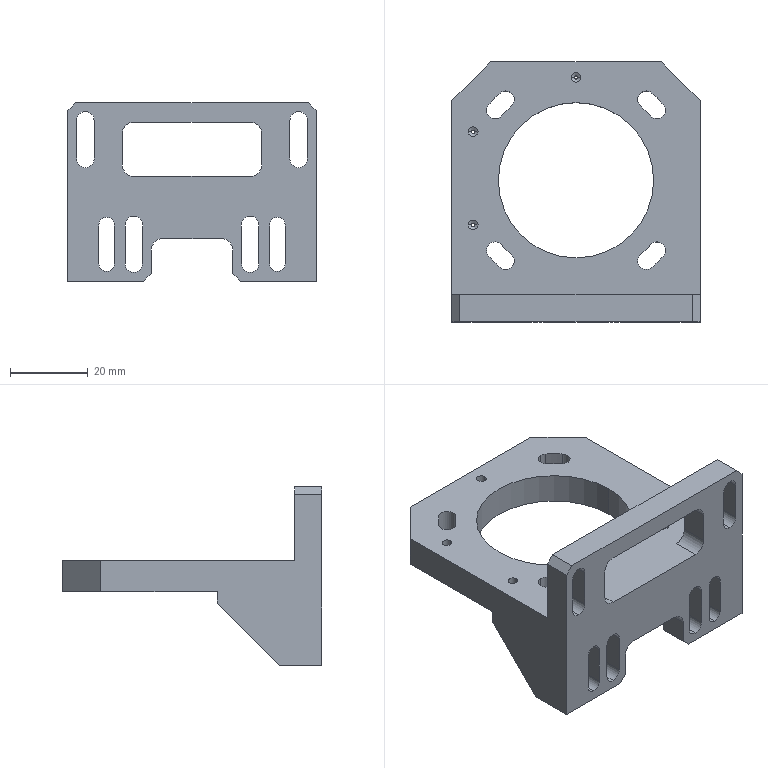NC program | NX | posted with a generic post | part box 64 x 67 x 46 mm
Lines 23993 to 24898 of 30645:
(ZLEVEL_PROFILE_COPY_2 , TOOL : D6JING)
N47966 T06 M6
N47968 G54
N47970 G17 G0 G90 X-21.427 Y23.915 B0. C0. S5000 M3
N47972 G43 Z30. H6
N47974 Z-0.1
N47976 G94 G1 X-21.88 Y24.7 F1000.
N47978 G3 X-22.4 Y25. R0.6
N47980 G1 X-23.5 F1500.
N47982 Y22.866
N47984 G3 X-23.2 Y22.346 R0.6
N47986 G1 X-22.3 Y21.827
N47988 G0 X-21.327 Y23.915 Z-0.2
N47990 G1 X-21.78 Y24.7 F1000.
N47992 G3 X-22.3 Y25. R0.6
N47994 G1 X-23.5 F1500.
N47996 Y22.849
N47998 G3 X-23.2 Y22.329 R0.6
N48000 G1 X-22.3 Y21.81
N48002 G0 X-21.227 Y23.914 Z-0.3
N48004 G1 X-21.68 Y24.7 F1000.
N48006 G3 X-22.2 Y25. R0.6
N48008 G1 X-23.5 F1500.
N48010 Y22.834
N48012 G3 X-23.2 Y22.314 R0.6
N48014 G1 X-22.3 Y21.794
N48016 G0 X-21.127 Y23.915 Z-0.4
N48018 G1 X-21.58 Y24.7 F1000.
N48020 G3 X-22.1 Y25. R0.6
N48022 G1 X-23.5 F1500.
N48024 Y22.82
N48026 G3 X-23.2 Y22.301 R0.6
N48028 G1 X-22.3 Y21.781
N48030 G0 X-21.027 Y23.914 Z-0.5
N48032 G1 X-21.48 Y24.7 F1000.
N48034 G3 X-22. Y25. R0.6
N48036 G1 X-23.5 F1500.
N48038 Y22.81
N48040 G3 X-23.2 Y22.29 R0.6
N48042 G1 X-22.3 Y21.77
N48044 G0 X-20.927 Y23.914 Z-0.6
N48046 G1 X-21.38 Y24.7 F1000.
N48048 G3 X-21.9 Y25. R0.6
N48050 G1 X-23.5 F1500.
N48052 Y22.803
N48054 G3 X-23.2 Y22.283 R0.6
N48056 G1 X-22.3 Y21.764
N48058 G0 X-20.827 Y23.914 Z-0.7
N48060 G1 X-21.28 Y24.7 F1000.
N48062 G3 X-21.8 Y25. R0.6
N48064 G1 X-23.5 F1500.
N48066 Y22.794
N48068 G3 X-23.2 Y22.274 R0.6
N48070 G1 X-22.3 Y21.755
N48072 G0 X-20.727 Y23.915 Z-0.8
N48074 G1 X-21.18 Y24.7 F1000.
N48076 G3 X-21.7 Y25. R0.6
N48078 G1 X-23.5 F1500.
N48080 Y22.789
N48082 G3 X-23.2 Y22.27 R0.6
N48084 G1 X-22.3 Y21.75
N48086 G0 X-20.627 Y23.914 Z-0.9
N48088 G1 X-21.08 Y24.7 F1000.
N48090 G3 X-21.6 Y25. R0.6
N48092 G1 X-23.5 F1500.
N48094 Y22.785
N48096 G3 X-23.2 Y22.265 R0.6
N48098 G1 X-22.3 Y21.746
N48100 G0 X-20.527 Y23.914 Z-1.
N48102 G1 X-20.98 Y24.7 F1000.
N48104 G3 X-21.5 Y25. R0.6
N48106 G1 X-23.5 F1500.
N48108 Y22.785
N48110 G3 X-23.2 Y22.265 R0.6
N48112 G1 X-22.3 Y21.745
N48114 G0 X-20.427 Y23.915 Z-1.1
N48116 G1 X-20.88 Y24.7 F1000.
N48118 G3 X-21.4 Y25. R0.6
N48120 G1 X-23.5 F1500.
N48122 Y22.785
N48124 G3 X-23.2 Y22.265 R0.6
N48126 G1 X-22.3 Y21.745
N48128 G0 X-20.327 Y23.914 Z-1.2
N48130 G1 X-20.78 Y24.7 F1000.
N48132 G3 X-21.3 Y25. R0.6
N48134 G1 X-23.5 F1500.
N48136 Y22.785
N48138 G3 X-23.2 Y22.265 R0.6
N48140 G1 X-22.3 Y21.745
N48142 G0 X-20.307 Y23.896 Z-1.3
N48144 G1 X-20.771 Y24.7 F1000.
N48146 G3 X-21.291 Y25. R0.6
N48148 G1 X-23.5 F1500.
N48150 Y22.785
N48152 G3 X-23.2 Y22.265 R0.6
N48154 G1 X-22.3 Y21.745
N48156 G0 X-20.296 Y23.878 Z-1.4
N48158 G1 X-20.771 Y24.7 F1000.
N48160 G3 X-21.291 Y25. R0.6
N48162 G1 X-23.5 F1500.
N48164 Y22.785
N48166 G3 X-23.2 Y22.265 R0.6
N48168 G1 X-22.3 Y21.745
N48170 G0 X-20.287 Y23.861 Z-1.5
N48172 G1 X-20.771 Y24.7 F1000.
N48174 G3 X-21.291 Y25. R0.6
N48176 G1 X-23.5 F1500.
N48178 Y22.785
N48180 G3 X-23.2 Y22.265 R0.6
N48182 G1 X-22.3 Y21.745
N48184 G0 X-20.278 Y23.846 Z-1.6
N48186 G1 X-20.771 Y24.7 F1000.
N48188 G3 X-21.291 Y25. R0.6
N48190 G1 X-23.5 F1500.
N48192 Y22.785
N48194 G3 X-23.2 Y22.265 R0.6
N48196 G1 X-22.3 Y21.745
N48198 G0 X-20.271 Y23.833 Z-1.7
N48200 G1 X-20.771 Y24.7 F1000.
N48202 G3 X-21.291 Y25. R0.6
N48204 G1 X-23.5 F1500.
N48206 Y22.785
N48208 G3 X-23.2 Y22.265 R0.6
N48210 G1 X-22.3 Y21.745
N48212 G0 X-20.265 Y23.823 Z-1.8
N48214 G1 X-20.771 Y24.7 F1000.
N48216 G3 X-21.291 Y25. R0.6
N48218 G1 X-23.5 F1500.
N48220 Y22.785
N48222 G3 X-23.2 Y22.265 R0.6
N48224 G1 X-22.3 Y21.745
N48226 G0 X-20.259 Y23.814 Z-1.9
N48228 G1 X-20.771 Y24.7 F1000.
N48230 G3 X-21.291 Y25. R0.6
N48232 G1 X-23.5 F1500.
N48234 Y22.785
N48236 G3 X-23.2 Y22.265 R0.6
N48238 G1 X-22.3 Y21.745
N48240 G0 X-20.255 Y23.807 Z-2.
N48242 G1 X-20.771 Y24.7 F1000.
N48244 G3 X-21.291 Y25. R0.6
N48246 G1 X-23.5 F1500.
N48248 Y22.785
N48250 G3 X-23.2 Y22.265 R0.6
N48252 G1 X-22.3 Y21.745
N48254 G0 X-20.253 Y23.803 Z-2.1
N48256 G1 X-20.771 Y24.7 F1000.
N48258 G3 X-21.291 Y25. R0.6
N48260 G1 X-23.5 F1500.
N48262 Y22.785
N48264 G3 X-23.2 Y22.265 R0.6
N48266 G1 X-22.3 Y21.745
N48268 G0 X-20.251 Y23.8 Z-2.2
N48270 G1 X-20.771 Y24.7 F1000.
N48272 G3 X-21.29 Y25. R0.6
N48274 G1 X-23.5 F1500.
N48276 Y22.785
N48278 G3 X-23.2 Y22.265 R0.6
N48280 G1 X-22.3 Y21.745
N48282 G0 X-20.251 Y23.8 Z-2.3
N48284 G1 X-20.771 Y24.7 F1000.
N48286 G3 X-21.29 Y25. R0.6
N48288 G1 X-23.5 F1500.
N48290 Y22.785
N48292 G3 X-23.2 Y22.265 R0.6
N48294 G1 X-22.3 Y21.745
N48296 G0 X-20.251 Y23.8 Z-2.4
N48298 G1 X-20.771 Y24.7 F1000.
N48300 G3 X-21.29 Y25. R0.6
N48302 G1 X-23.5 F1500.
N48304 Y22.785
N48306 G3 X-23.2 Y22.265 R0.6
N48308 G1 X-22.3 Y21.745
N48310 G0 X-20.251 Y23.8 Z-2.5
N48312 G1 X-20.771 Y24.7 F1000.
N48314 G3 X-21.29 Y25. R0.6
N48316 G1 X-23.5 F1500.
N48318 Y22.785
N48320 G3 X-23.2 Y22.265 R0.6
N48322 G1 X-22.3 Y21.745
N48324 G0 X-20.251 Y23.8 Z-2.6
N48326 G1 X-20.771 Y24.7 F1000.
N48328 G3 X-21.29 Y25. R0.6
N48330 G1 X-23.5 F1500.
N48332 Y22.785
N48334 G3 X-23.2 Y22.265 R0.6
N48336 G1 X-22.3 Y21.745
N48338 G0 X-20.251 Y23.8 Z-2.7
N48340 G1 X-20.771 Y24.7 F1000.
N48342 G3 X-21.29 Y25. R0.6
N48344 G1 X-23.5 F1500.
N48346 Y22.785
N48348 G3 X-23.2 Y22.265 R0.6
N48350 G1 X-22.3 Y21.745
N48352 G0 X-20.251 Y23.8 Z-2.8
N48354 G1 X-20.771 Y24.7 F1000.
N48356 G3 X-21.29 Y25. R0.6
N48358 G1 X-23.5 F1500.
N48360 Y22.784
N48362 G3 X-23.2 Y22.265 R0.6
N48364 G1 X-22.3 Y21.745
N48366 G0 X-20.251 Y23.8 Z-2.9
N48368 G1 X-20.77 Y24.7 F1000.
N48370 G3 X-21.29 Y25. R0.6
N48372 G1 X-23.5 F1500.
N48374 Y22.784
N48376 G3 X-23.2 Y22.265 R0.6
N48378 G1 X-22.3 Y21.745
N48380 G0 X-20.251 Y23.8 Z-3.
N48382 G1 X-20.77 Y24.7 F1000.
N48384 G3 X-21.29 Y25. R0.6
N48386 G1 X-23.5 F1500.
N48388 Y22.784
N48390 G3 X-23.2 Y22.265 R0.6
N48392 G1 X-22.3 Y21.745
N48394 G0 X-20.251 Y23.8 Z-3.1
N48396 G1 X-20.77 Y24.7 F1000.
N48398 G3 X-21.29 Y25. R0.6
N48400 G1 X-23.5 F1500.
N48402 Y22.784
N48404 G3 X-23.2 Y22.265 R0.6
N48406 G1 X-22.3 Y21.745
N48408 G0 X-20.251 Y23.8 Z-3.2
N48410 G1 X-20.77 Y24.7 F1000.
N48412 G3 X-21.29 Y25. R0.6
N48414 G1 X-23.5 F1500.
N48416 Y22.784
N48418 G3 X-23.2 Y22.265 R0.6
N48420 G1 X-22.3 Y21.745
N48422 G0 X-20.251 Y23.8 Z-3.3
N48424 G1 X-20.77 Y24.7 F1000.
N48426 G3 X-21.29 Y25. R0.6
N48428 G1 X-23.5 F1500.
N48430 Y22.784
N48432 G3 X-23.2 Y22.265 R0.6
N48434 G1 X-22.3 Y21.745
N48436 G0 X-20.251 Y23.8 Z-3.4
N48438 G1 X-20.77 Y24.7 F1000.
N48440 G3 X-21.29 Y25. R0.6
N48442 G1 X-23.5 F1500.
N48444 Y22.784
N48446 G3 X-23.2 Y22.265 R0.6
N48448 G1 X-22.3 Y21.745
N48450 G0 X-20.251 Y23.8 Z-3.5
N48452 G1 X-20.77 Y24.7 F1000.
N48454 G3 X-21.29 Y25. R0.6
N48456 G1 X-23.5 F1500.
N48458 Y22.784
N48460 G3 X-23.2 Y22.265 R0.6
N48462 G1 X-22.3 Y21.745
N48464 G0 X-20.25 Y23.8 Z-3.6
N48466 G1 X-20.77 Y24.7 F1000.
N48468 G3 X-21.29 Y25. R0.6
N48470 G1 X-23.5 F1500.
N48472 Y22.784
N48474 G3 X-23.2 Y22.265 R0.6
N48476 G1 X-22.3 Y21.745
N48478 G0 X-20.25 Y23.8 Z-3.7
N48480 G1 X-20.77 Y24.7 F1000.
N48482 G3 X-21.29 Y25. R0.6
N48484 G1 X-23.5 F1500.
N48486 Y22.784
N48488 G3 X-23.2 Y22.265 R0.6
N48490 G1 X-22.3 Y21.745
N48492 G0 X-20.25 Y23.8 Z-3.8
N48494 G1 X-20.77 Y24.7 F1000.
N48496 G3 X-21.29 Y25. R0.6
N48498 G1 X-23.5 F1500.
N48500 Y22.784
N48502 G3 X-23.2 Y22.265 R0.6
N48504 G1 X-22.3 Y21.745
N48506 G0 X-20.25 Y23.8 Z-3.9
N48508 G1 X-20.77 Y24.7 F1000.
N48510 G3 X-21.29 Y25. R0.6
N48512 G1 X-23.5 F1500.
N48514 Y22.784
N48516 G3 X-23.2 Y22.265 R0.6
N48518 G1 X-22.3 Y21.745
N48520 G0 X-20.25 Y23.8 Z-4.
N48522 G1 X-20.77 Y24.7 F1000.
N48524 G3 X-21.29 Y25. R0.6
N48526 G1 X-23.5 F1500.
N48528 Y22.784
N48530 G3 X-23.2 Y22.265 R0.6
N48532 G1 X-22.3 Y21.745
N48534 G0 X-20.25 Y23.8 Z-4.1
N48536 G1 X-20.77 Y24.7 F1000.
N48538 G3 X-21.289 Y25. R0.6
N48540 G1 X-23.5 F1500.
N48542 Y22.784
N48544 G3 X-23.2 Y22.265 R0.6
N48546 G1 X-22.3 Y21.745
N48548 G0 X-20.25 Y23.8 Z-4.2
N48550 G1 X-20.77 Y24.7 F1000.
N48552 G3 X-21.289 Y25. R0.6
N48554 G1 X-23.5 F1500.
N48556 Y22.784
N48558 G3 X-23.2 Y22.265 R0.6
N48560 G1 X-22.3 Y21.745
N48562 G0 X-20.25 Y23.8 Z-4.3
N48564 G1 X-20.77 Y24.7 F1000.
N48566 G3 X-21.289 Y25. R0.6
N48568 G1 X-23.5 F1500.
N48570 Y22.784
N48572 G3 X-23.2 Y22.265 R0.6
N48574 G1 X-22.3 Y21.745
N48576 G0 X-20.25 Y23.8 Z-4.4
N48578 G1 X-20.77 Y24.7 F1000.
N48580 G3 X-21.289 Y25. R0.6
N48582 G1 X-23.5 F1500.
N48584 Y22.784
N48586 G3 X-23.2 Y22.265 R0.6
N48588 G1 X-22.3 Y21.745
N48590 G0 X-20.25 Y23.8 Z-4.5
N48592 G1 X-20.77 Y24.7 F1000.
N48594 G3 X-21.289 Y25. R0.6
N48596 G1 X-23.5 F1500.
N48598 Y22.784
N48600 G3 X-23.2 Y22.265 R0.6
N48602 G1 X-22.3 Y21.745
N48604 G0 X-20.25 Y23.8 Z-4.6
N48606 G1 X-20.77 Y24.7 F1000.
N48608 G3 X-21.289 Y25. R0.6
N48610 G1 X-23.5 F1500.
N48612 Y22.784
N48614 G3 X-23.2 Y22.265 R0.6
N48616 G1 X-22.3 Y21.745
N48618 G0 X-20.25 Y23.8 Z-4.7
N48620 G1 X-20.77 Y24.7 F1000.
N48622 G3 X-21.289 Y25. R0.6
N48624 G1 X-23.5 F1500.
N48626 Y22.784
N48628 G3 X-23.2 Y22.265 R0.6
N48630 G1 X-22.3 Y21.745
N48632 G0 X-20.25 Y23.8 Z-4.8
N48634 G1 X-20.769 Y24.7 F1000.
N48636 G3 X-21.289 Y25. R0.6
N48638 G1 X-23.5 F1500.
N48640 Y22.784
N48642 G3 X-23.2 Y22.265 R0.6
N48644 G1 X-22.3 Y21.745
N48646 G0 X-20.25 Y23.8 Z-4.9
N48648 G1 X-20.769 Y24.7 F1000.
N48650 G3 X-21.289 Y25. R0.6
N48652 G1 X-23.5 F1500.
N48654 Y22.784
N48656 G3 X-23.2 Y22.265 R0.6
N48658 G1 X-22.3 Y21.745
N48660 G0 X-20.25 Y23.8 Z-5.
N48662 G1 X-20.769 Y24.7 F1000.
N48664 G3 X-21.289 Y25. R0.6
N48666 G1 X-23.5 F1500.
N48668 Y22.784
N48670 G3 X-23.2 Y22.265 R0.6
N48672 G1 X-22.3 Y21.745
N48674 G0 X-20.25 Y23.8 Z-5.1
N48676 G1 X-20.769 Y24.7 F1000.
N48678 G3 X-21.289 Y25. R0.6
N48680 G1 X-23.5 F1500.
N48682 Y22.784
N48684 G3 X-23.2 Y22.265 R0.6
N48686 G1 X-22.3 Y21.745
N48688 G0 X-20.25 Y23.8 Z-5.2
N48690 G1 X-20.769 Y24.7 F1000.
N48692 G3 X-21.289 Y25. R0.6
N48694 G1 X-23.5 F1500.
N48696 Y22.784
N48698 G3 X-23.2 Y22.265 R0.6
N48700 G1 X-22.3 Y21.745
N48702 G0 X-20.25 Y23.8 Z-5.3
N48704 G1 X-20.769 Y24.7 F1000.
N48706 G3 X-21.289 Y25. R0.6
N48708 G1 X-23.5 F1500.
N48710 Y22.784
N48712 G3 X-23.2 Y22.265 R0.6
N48714 G1 X-22.3 Y21.745
N48716 G0 X-20.25 Y23.8 Z-5.4
N48718 G1 X-20.769 Y24.7 F1000.
N48720 G3 X-21.289 Y25. R0.6
N48722 G1 X-23.5 F1500.
N48724 Y22.784
N48726 G3 X-23.2 Y22.265 R0.6
N48728 G1 X-22.3 Y21.745
N48730 G0 X-20.249 Y23.8 Z-5.5
N48732 G1 X-20.769 Y24.7 F1000.
N48734 G3 X-21.289 Y25. R0.6
N48736 G1 X-23.5 F1500.
N48738 Y22.784
N48740 G3 X-23.2 Y22.265 R0.6
N48742 G1 X-22.3 Y21.745
N48744 G0 X-20.249 Y23.8 Z-5.6
N48746 G1 X-20.769 Y24.7 F1000.
N48748 G3 X-21.289 Y25. R0.6
N48750 G1 X-23.5 F1500.
N48752 Y22.784
N48754 G3 X-23.2 Y22.265 R0.6
N48756 G1 X-22.3 Y21.745
N48758 G0 X-20.249 Y23.8 Z-5.7
N48760 G1 X-20.769 Y24.7 F1000.
N48762 G3 X-21.289 Y25. R0.6
N48764 G1 X-23.5 F1500.
N48766 Y22.784
N48768 G3 X-23.2 Y22.265 R0.6
N48770 G1 X-22.3 Y21.745
N48772 G0 X-20.249 Y23.8 Z-5.8
N48774 G1 X-20.769 Y24.7 F1000.
N48776 G3 X-21.289 Y25. R0.6
N48778 G1 X-23.5 F1500.
N48780 Y22.784
N48782 G3 X-23.2 Y22.265 R0.6
N48784 G1 X-22.3 Y21.745
N48786 G0 X-20.249 Y23.8 Z-5.9
N48788 G1 X-20.769 Y24.7 F1000.
N48790 G3 X-21.288 Y25. R0.6
N48792 G1 X-23.5 F1500.
N48794 Y22.784
N48796 G3 X-23.2 Y22.265 R0.6
N48798 G1 X-22.3 Y21.745
N48800 G0 X-20.249 Y23.8 Z-6.
N48802 G1 X-20.769 Y24.7 F1000.
N48804 G3 X-21.288 Y25. R0.6
N48806 G1 X-23.5 F1500.
N48808 Y22.784
N48810 G3 X-23.2 Y22.265 R0.6
N48812 G1 X-22.3 Y21.745
N48814 G0 X-20.249 Y23.8 Z-6.1
N48816 G1 X-20.769 Y24.7 F1000.
N48818 G3 X-21.288 Y25. R0.6
N48820 G1 X-23.5 F1500.
N48822 Y22.784
N48824 G3 X-23.2 Y22.265 R0.6
N48826 G1 X-22.3 Y21.745
N48828 G0 X-20.249 Y23.8 Z-6.2
N48830 G1 X-20.769 Y24.7 F1000.
N48832 G3 X-21.288 Y25. R0.6
N48834 G1 X-23.5 F1500.
N48836 Y22.784
N48838 G3 X-23.2 Y22.265 R0.6
N48840 G1 X-22.3 Y21.745
N48842 G0 X-20.249 Y23.8 Z-6.3
N48844 G1 X-20.769 Y24.7 F1000.
N48846 G3 X-21.288 Y25. R0.6
N48848 G1 X-23.5 F1500.
N48850 Y22.784
N48852 G3 X-23.2 Y22.265 R0.6
N48854 G1 X-22.3 Y21.745
N48856 G0 X-20.249 Y23.8 Z-6.4
N48858 G1 X-20.769 Y24.7 F1000.
N48860 G3 X-21.288 Y25. R0.6
N48862 G1 X-23.5 F1500.
N48864 Y22.784
N48866 G3 X-23.2 Y22.265 R0.6
N48868 G1 X-22.3 Y21.745
N48870 G0 X-20.249 Y23.8 Z-6.5
N48872 G1 X-20.769 Y24.7 F1000.
N48874 G3 X-21.288 Y25. R0.6
N48876 G1 X-23.5 F1500.
N48878 Y22.784
N48880 G3 X-23.2 Y22.265 R0.6
N48882 G1 X-22.3 Y21.745
N48884 G0 X-20.249 Y23.8 Z-6.6
N48886 G1 X-20.768 Y24.7 F1000.
N48888 G3 X-21.288 Y25. R0.6
N48890 G1 X-23.5 F1500.
N48892 Y22.784
N48894 G3 X-23.2 Y22.265 R0.6
N48896 G1 X-22.3 Y21.745
N48898 G0 X-20.249 Y23.8 Z-6.7
N48900 G1 X-20.768 Y24.7 F1000.
N48902 G3 X-21.288 Y25. R0.6
N48904 G1 X-23.5 F1500.
N48906 Y22.784
N48908 G3 X-23.2 Y22.265 R0.6
N48910 G1 X-22.3 Y21.745
N48912 G0 X-20.249 Y23.8 Z-6.8
N48914 G1 X-20.768 Y24.7 F1000.
N48916 G3 X-21.288 Y25. R0.6
N48918 G1 X-23.5 F1500.
N48920 Y22.784
N48922 G3 X-23.2 Y22.265 R0.6
N48924 G1 X-22.3 Y21.745
N48926 G0 X-20.249 Y23.8 Z-6.9
N48928 G1 X-20.768 Y24.7 F1000.
N48930 G3 X-21.288 Y25. R0.6
N48932 G1 X-23.5 F1500.
N48934 Y22.784
N48936 G3 X-23.2 Y22.265 R0.6
N48938 G1 X-22.3 Y21.745
N48940 G0 X-20.249 Y23.8 Z-7.
N48942 G1 X-20.768 Y24.7 F1000.
N48944 G3 X-21.288 Y25. R0.6
N48946 G1 X-23.5 F1500.
N48948 Y22.784
N48950 G3 X-23.2 Y22.265 R0.6
N48952 G1 X-22.3 Y21.745
N48954 G0 X-20.249 Y23.8 Z-7.1
N48956 G1 X-20.768 Y24.7 F1000.
N48958 G3 X-21.288 Y25. R0.6
N48960 G1 X-23.5 F1500.
N48962 Y22.784
N48964 G3 X-23.2 Y22.265 R0.6
N48966 G1 X-22.3 Y21.745
N48968 G0 X-20.249 Y23.8 Z-7.2
N48970 G1 X-20.768 Y24.7 F1000.
N48972 G3 X-21.288 Y25. R0.6
N48974 G1 X-23.5 F1500.
N48976 Y22.784
N48978 G3 X-23.2 Y22.265 R0.6
N48980 G1 X-22.3 Y21.745
N48982 G0 X-20.248 Y23.8 Z-7.3
N48984 G1 X-20.768 Y24.7 F1000.
N48986 G3 X-21.288 Y25. R0.6
N48988 G1 X-23.5 F1500.
N48990 Y22.784
N48992 G3 X-23.2 Y22.265 R0.6
N48994 G1 X-22.3 Y21.745
N48996 G0 X-20.248 Y23.8 Z-7.4
N48998 G1 X-20.768 Y24.7 F1000.
N49000 G3 X-21.288 Y25. R0.6
N49002 G1 X-23.5 F1500.
N49004 Y22.784
N49006 G3 X-23.2 Y22.265 R0.6
N49008 G1 X-22.3 Y21.745
N49010 G0 X-20.248 Y23.8 Z-7.5
N49012 G1 X-20.768 Y24.7 F1000.
N49014 G3 X-21.288 Y25. R0.6
N49016 G1 X-23.5 F1500.
N49018 Y22.784
N49020 G3 X-23.2 Y22.265 R0.6
N49022 G1 X-22.3 Y21.745
N49024 G0 X-20.248 Y23.8 Z-7.6
N49026 G1 X-20.768 Y24.7 F1000.
N49028 G3 X-21.288 Y25. R0.6
N49030 G1 X-23.5 F1500.
N49032 Y22.784
N49034 G3 X-23.2 Y22.265 R0.6
N49036 G1 X-22.3 Y21.745
N49038 G0 X-20.248 Y23.8 Z-7.7
N49040 G1 X-20.768 Y24.7 F1000.
N49042 G3 X-21.288 Y25. R0.6
N49044 G1 X-23.5 F1500.
N49046 Y22.784
N49048 G3 X-23.2 Y22.264 R0.6
N49050 G1 X-22.3 Y21.745
N49052 G0 X-20.248 Y23.8 Z-7.8
N49054 G1 X-20.768 Y24.7 F1000.
N49056 G3 X-21.287 Y25. R0.6
N49058 G1 X-23.5 F1500.
N49060 Y22.784
N49062 G3 X-23.2 Y22.264 R0.6
N49064 G1 X-22.3 Y21.745
N49066 G0 X-20.248 Y23.8 Z-7.9
N49068 G1 X-20.768 Y24.7 F1000.
N49070 G3 X-21.287 Y25. R0.6
N49072 G1 X-23.5 F1500.
N49074 Y22.784
N49076 G3 X-23.2 Y22.264 R0.6
N49078 G1 X-22.3 Y21.745
N49080 G0 X-20.248 Y23.8 Z-8.
N49082 G1 X-20.768 Y24.7 F1000.
N49084 G3 X-21.287 Y25. R0.6
N49086 G1 X-23.5 F1500.
N49088 Y22.784
N49090 G3 X-23.2 Y22.264 R0.6
N49092 G1 X-22.3 Y21.745
N49094 G0 X-20.248 Y23.8 Z-8.1
N49096 G1 X-20.768 Y24.7 F1000.
N49098 G3 X-21.287 Y25. R0.6
N49100 G1 X-23.5 F1500.
N49102 Y22.784
N49104 G3 X-23.2 Y22.264 R0.6
N49106 G1 X-22.3 Y21.745
N49108 G0 X-20.248 Y23.8 Z-8.2
N49110 G1 X-20.768 Y24.7 F1000.
N49112 G3 X-21.287 Y25. R0.6
N49114 G1 X-23.5 F1500.
N49116 Y22.784
N49118 G3 X-23.2 Y22.264 R0.6
N49120 G1 X-22.3 Y21.745
N49122 G0 X-20.248 Y23.8 Z-8.3
N49124 G1 X-20.768 Y24.7 F1000.
N49126 G3 X-21.287 Y25. R0.6
N49128 G1 X-23.5 F1500.
N49130 Y22.784
N49132 G3 X-23.2 Y22.264 R0.6
N49134 G1 X-22.3 Y21.745
N49136 G0 X-20.248 Y23.8 Z-8.4
N49138 G1 X-20.768 Y24.7 F1000.
N49140 G3 X-21.287 Y25. R0.6
N49142 G1 X-23.5 F1500.
N49144 Y22.784
N49146 G3 X-23.2 Y22.264 R0.6
N49148 G1 X-22.3 Y21.745
N49150 G0 X-20.248 Y23.8 Z-8.5
N49152 G1 X-20.767 Y24.7 F1000.
N49154 G3 X-21.287 Y25. R0.6
N49156 G1 X-23.5 F1500.
N49158 Y22.784
N49160 G3 X-23.2 Y22.264 R0.6
N49162 G1 X-22.3 Y21.745
N49164 G0 X-20.248 Y23.8 Z-8.6
N49166 G1 X-20.767 Y24.7 F1000.
N49168 G3 X-21.287 Y25. R0.6
N49170 G1 X-23.5 F1500.
N49172 Y22.784
N49174 G3 X-23.2 Y22.264 R0.6
N49176 G1 X-22.3 Y21.745
N49178 G0 X-20.248 Y23.8 Z-8.7
N49180 G1 X-20.767 Y24.7 F1000.
N49182 G3 X-21.287 Y25. R0.6
N49184 G1 X-23.5 F1500.
N49186 Y22.784
N49188 G3 X-23.2 Y22.264 R0.6
N49190 G1 X-22.3 Y21.745
N49192 G0 X-20.248 Y23.8 Z-8.8
N49194 G1 X-20.767 Y24.7 F1000.
N49196 G3 X-21.287 Y25. R0.6
N49198 G1 X-23.5 F1500.
N49200 Y22.784
N49202 G3 X-23.2 Y22.264 R0.6
N49204 G1 X-22.3 Y21.745
N49206 G0 X-20.248 Y23.8 Z-8.9
N49208 G1 X-20.767 Y24.7 F1000.
N49210 G3 X-21.287 Y25. R0.6
N49212 G1 X-23.5 F1500.
N49214 Y22.784
N49216 G3 X-23.2 Y22.264 R0.6
N49218 G1 X-22.3 Y21.745
N49220 G0 X-20.248 Y23.8 Z-9.
N49222 G1 X-20.767 Y24.7 F1000.
N49224 G3 X-21.287 Y25. R0.6
N49226 G1 X-23.5 F1500.
N49228 Y22.784
N49230 G3 X-23.2 Y22.264 R0.6
N49232 G1 X-22.3 Y21.745
N49234 G0 X-20.248 Y23.8 Z-9.1
N49236 G1 X-20.767 Y24.7 F1000.
N49238 G3 X-21.287 Y25. R0.6
N49240 G1 X-23.5 F1500.
N49242 Y22.784
N49244 G3 X-23.2 Y22.264 R0.6
N49246 G1 X-22.3 Y21.745
N49248 G0 X-20.247 Y23.8 Z-9.2
N49250 G1 X-20.767 Y24.7 F1000.
N49252 G3 X-21.287 Y25. R0.6
N49254 G1 X-23.5 F1500.
N49256 Y22.784
N49258 G3 X-23.2 Y22.264 R0.6
N49260 G1 X-22.3 Y21.745
N49262 G0 X-20.247 Y23.8 Z-9.3
N49264 G1 X-20.767 Y24.7 F1000.
N49266 G3 X-21.287 Y25. R0.6
N49268 G1 X-23.5 F1500.
N49270 Y22.784
N49272 G3 X-23.2 Y22.264 R0.6
N49274 G1 X-22.3 Y21.745
N49276 G0 X-20.247 Y23.8 Z-9.4
N49278 G1 X-20.767 Y24.7 F1000.
N49280 G3 X-21.287 Y25. R0.6
N49282 G1 X-23.5 F1500.
N49284 Y22.784
N49286 G3 X-23.2 Y22.264 R0.6
N49288 G1 X-22.3 Y21.745
N49290 G0 X-20.247 Y23.8 Z-9.5
N49292 G1 X-20.767 Y24.7 F1000.
N49294 G3 X-21.287 Y25. R0.6
N49296 G1 X-23.5 F1500.
N49298 Y22.784
N49300 G3 X-23.2 Y22.264 R0.6
N49302 G1 X-22.3 Y21.745
N49304 G0 X-20.247 Y23.8 Z-9.6
N49306 G1 X-20.767 Y24.7 F1000.
N49308 G3 X-21.286 Y25. R0.6
N49310 G1 X-23.5 F1500.
N49312 Y22.784
N49314 G3 X-23.2 Y22.264 R0.6
N49316 G1 X-22.3 Y21.745
N49318 G0 X-20.247 Y23.8 Z-9.7
N49320 G1 X-20.767 Y24.7 F1000.
N49322 G3 X-21.286 Y25. R0.6
N49324 G1 X-23.5 F1500.
N49326 Y22.784
N49328 G3 X-23.2 Y22.264 R0.6
N49330 G1 X-22.3 Y21.745
N49332 G0 X-20.247 Y23.8 Z-9.8
N49334 G1 X-20.767 Y24.7 F1000.
N49336 G3 X-21.286 Y25. R0.6
N49338 G1 X-23.5 F1500.
N49340 Y22.784
N49342 G3 X-23.2 Y22.264 R0.6
N49344 G1 X-22.3 Y21.745
N49346 G0 X-20.247 Y23.8 Z-9.9
N49348 G1 X-20.767 Y24.7 F1000.
N49350 G3 X-21.286 Y25. R0.6
N49352 G1 X-23.5 F1500.
N49354 Y22.784
N49356 G3 X-23.2 Y22.264 R0.6
N49358 G1 X-22.3 Y21.745
N49360 G0 X-20.247 Y23.8 Z-10.
N49362 G1 X-20.767 Y24.7 F1000.
N49364 G3 X-21.286 Y25. R0.6
N49366 G1 X-23.5 F1500.
N49368 Y22.784
N49370 G3 X-23.2 Y22.264 R0.6
N49372 G1 X-22.3 Y21.745
N49374 G0 X-20.247 Y23.8 Z-10.1
N49376 G1 X-20.767 Y24.7 F1000.
N49378 G3 X-21.286 Y25. R0.6
N49380 G1 X-23.5 F1500.
N49382 Y22.784
N49384 G3 X-23.2 Y22.264 R0.6
N49386 G1 X-22.3 Y21.745
N49388 G0 X-20.247 Y23.8 Z-10.2
N49390 G1 X-20.767 Y24.7 F1000.
N49392 G3 X-21.286 Y25. R0.6
N49394 G1 X-23.5 F1500.
N49396 Y22.784
N49398 G3 X-23.2 Y22.264 R0.6
N49400 G1 X-22.3 Y21.745
N49402 G0 X-20.247 Y23.8 Z-10.3
N49404 G1 X-20.766 Y24.7 F1000.
N49406 G3 X-21.286 Y25. R0.6
N49408 G1 X-23.5 F1500.
N49410 Y22.784
N49412 G3 X-23.2 Y22.264 R0.6
N49414 G1 X-22.3 Y21.745
N49416 G0 X-20.247 Y23.8 Z-10.4
N49418 G1 X-20.766 Y24.7 F1000.
N49420 G3 X-21.286 Y25. R0.6
N49422 G1 X-23.5 F1500.
N49424 Y22.784
N49426 G3 X-23.2 Y22.264 R0.6
N49428 G1 X-22.3 Y21.745
N49430 G0 X-20.247 Y23.8 Z-10.5
N49432 G1 X-20.766 Y24.7 F1000.
N49434 G3 X-21.286 Y25. R0.6
N49436 G1 X-23.5 F1500.
N49438 Y22.784
N49440 G3 X-23.2 Y22.264 R0.6
N49442 G1 X-22.3 Y21.745
N49444 G0 X-20.247 Y23.8 Z-10.6
N49446 G1 X-20.766 Y24.7 F1000.
N49448 G3 X-21.286 Y25. R0.6
N49450 G1 X-23.5 F1500.
N49452 Y22.784
N49454 G3 X-23.2 Y22.264 R0.6
N49456 G1 X-22.3 Y21.745
N49458 G0 X-20.247 Y23.8 Z-10.7
N49460 G1 X-20.766 Y24.7 F1000.
N49462 G3 X-21.286 Y25. R0.6
N49464 G1 X-23.5 F1500.
N49466 Y22.784
N49468 G3 X-23.2 Y22.264 R0.6
N49470 G1 X-22.3 Y21.745
N49472 G0 X-20.247 Y23.8 Z-10.8
N49474 G1 X-20.766 Y24.7 F1000.
N49476 G3 X-21.286 Y25. R0.6
N49478 G1 X-23.5 F1500.
N49480 Y22.784
N49482 G3 X-23.2 Y22.264 R0.6
N49484 G1 X-22.3 Y21.745
N49486 G0 X-20.247 Y23.8 Z-10.9
N49488 G1 X-20.766 Y24.7 F1000.
N49490 G3 X-21.286 Y25. R0.6
N49492 G1 X-23.5 F1500.
N49494 Y22.784
N49496 G3 X-23.2 Y22.264 R0.6
N49498 G1 X-22.3 Y21.745
N49500 G0 X-20.246 Y23.8 Z-11.
N49502 G1 X-20.766 Y24.7 F1000.
N49504 G3 X-21.286 Y25. R0.6
N49506 G1 X-23.5 F1500.
N49508 Y22.784
N49510 G3 X-23.2 Y22.264 R0.6
N49512 G1 X-22.3 Y21.745
N49514 G0 X-20.246 Y23.8 Z-11.1
N49516 G1 X-20.766 Y24.7 F1000.
N49518 G3 X-21.286 Y25. R0.6
N49520 G1 X-23.5 F1500.
N49522 Y22.784
N49524 G3 X-23.2 Y22.264 R0.6
N49526 G1 X-22.3 Y21.745
N49528 G0 X-20.246 Y23.8 Z-11.2
N49530 G1 X-20.766 Y24.7 F1000.
N49532 G3 X-21.286 Y25. R0.6
N49534 G1 X-23.5 F1500.
N49536 Y22.784
N49538 G3 X-23.2 Y22.264 R0.6
N49540 G1 X-22.3 Y21.745
N49542 G0 X-20.246 Y23.8 Z-11.3
N49544 G1 X-20.766 Y24.7 F1000.
N49546 G3 X-21.286 Y25. R0.6
N49548 G1 X-23.5 F1500.
N49550 Y22.784
N49552 G3 X-23.2 Y22.264 R0.6
N49554 G1 X-22.3 Y21.745
N49556 G0 X-20.246 Y23.8 Z-11.4
N49558 G1 X-20.766 Y24.7 F1000.
N49560 G3 X-21.285 Y25. R0.6
N49562 G1 X-23.5 F1500.
N49564 Y22.784
N49566 G3 X-23.2 Y22.264 R0.6
N49568 G1 X-22.3 Y21.745
N49570 G0 X-20.246 Y23.8 Z-11.5
N49572 G1 X-20.766 Y24.7 F1000.
N49574 G3 X-21.285 Y25. R0.6
N49576 G1 X-23.5 F1500.
N49578 Y22.784
N49580 G3 X-23.2 Y22.264 R0.6
N49582 G1 X-22.3 Y21.745
N49584 G0 X-20.246 Y23.8 Z-11.6
N49586 G1 X-20.766 Y24.7 F1000.
N49588 G3 X-21.285 Y25. R0.6
N49590 G1 X-23.5 F1500.
N49592 Y22.784
N49594 G3 X-23.2 Y22.264 R0.6
N49596 G1 X-22.3 Y21.745
N49598 G0 X-20.246 Y23.8 Z-11.7
N49600 G1 X-20.766 Y24.7 F1000.
N49602 G3 X-21.285 Y25. R0.6
N49604 G1 X-23.5 F1500.
N49606 Y22.784
N49608 G3 X-23.2 Y22.264 R0.6
N49610 G1 X-22.3 Y21.745
N49612 G0 X-20.246 Y23.8 Z-11.8
N49614 G1 X-20.766 Y24.7 F1000.
N49616 G3 X-21.285 Y25. R0.6
N49618 G1 X-23.5 F1500.
N49620 Y22.784
N49622 G3 X-23.2 Y22.264 R0.6
N49624 G1 X-22.3 Y21.745
N49626 G0 X-20.246 Y23.8 Z-11.9
N49628 G1 X-20.766 Y24.7 F1000.
N49630 G3 X-21.285 Y25. R0.6
N49632 G1 X-23.5 F1500.
N49634 Y22.784
N49636 G3 X-23.2 Y22.264 R0.6
N49638 G1 X-22.3 Y21.745
N49640 G0 X-20.246 Y23.8 Z-12.
N49642 G1 X-20.766 Y24.7 F1000.
N49644 G3 X-21.285 Y25. R0.6
N49646 G1 X-23.5 F1500.
N49648 Y22.784
N49650 G3 X-23.2 Y22.264 R0.6
N49652 G1 X-22.3 Y21.745
N49654 G0 X-20.246 Y23.8 Z-12.1
N49656 G1 X-20.765 Y24.7 F1000.
N49658 G3 X-21.285 Y25. R0.6
N49660 G1 X-23.5 F1500.
N49662 Y22.784
N49664 G3 X-23.2 Y22.264 R0.6
N49666 G1 X-22.3 Y21.745
N49668 G0 X-20.246 Y23.8 Z-12.2
N49670 G1 X-20.765 Y24.7 F1000.
N49672 G3 X-21.285 Y25. R0.6
N49674 G1 X-23.5 F1500.
N49676 Y22.784
N49678 G3 X-23.2 Y22.264 R0.6
N49680 G1 X-22.3 Y21.745
N49682 G0 X-20.246 Y23.8 Z-12.3
N49684 G1 X-20.765 Y24.7 F1000.
N49686 G3 X-21.285 Y25. R0.6
N49688 G1 X-23.5 F1500.
N49690 Y22.784
N49692 G3 X-23.2 Y22.264 R0.6
N49694 G1 X-22.3 Y21.745
N49696 G0 X-20.246 Y23.8 Z-12.4
N49698 G1 X-20.765 Y24.7 F1000.
N49700 G3 X-21.285 Y25. R0.6
N49702 G1 X-23.5 F1500.
N49704 Y22.784
N49706 G3 X-23.2 Y22.264 R0.6
N49708 G1 X-22.3 Y21.745
N49710 G0 X-20.246 Y23.8 Z-12.5
N49712 G1 X-20.765 Y24.7 F1000.
N49714 G3 X-21.285 Y25. R0.6
N49716 G1 X-23.5 F1500.
N49718 Y22.784
N49720 G3 X-23.2 Y22.264 R0.6
N49722 G1 X-22.3 Y21.745
N49724 G0 X-20.246 Y23.8 Z-12.6
N49726 G1 X-20.765 Y24.7 F1000.
N49728 G3 X-21.285 Y25. R0.6
N49730 G1 X-23.5 F1500.
N49732 Y22.784
N49734 G3 X-23.2 Y22.264 R0.6
N49736 G1 X-22.3 Y21.745
N49738 G0 X-20.246 Y23.8 Z-12.7
N49740 G1 X-20.765 Y24.7 F1000.
N49742 G3 X-21.285 Y25. R0.6
N49744 G1 X-23.5 F1500.
N49746 Y22.784
N49748 G3 X-23.2 Y22.264 R0.6
N49750 G1 X-22.3 Y21.744
N49752 G0 X-20.245 Y23.8 Z-12.8
N49754 G1 X-20.765 Y24.7 F1000.
N49756 G3 X-21.285 Y25. R0.6
N49758 G1 X-23.5 F1500.
N49760 Y22.784
N49762 G3 X-23.2 Y22.264 R0.6
N49764 G1 X-22.3 Y21.744
N49766 G0 X-20.245 Y23.8 Z-12.9
N49768 G1 X-20.765 Y24.7 F1000.
N49770 G3 X-21.285 Y25. R0.6